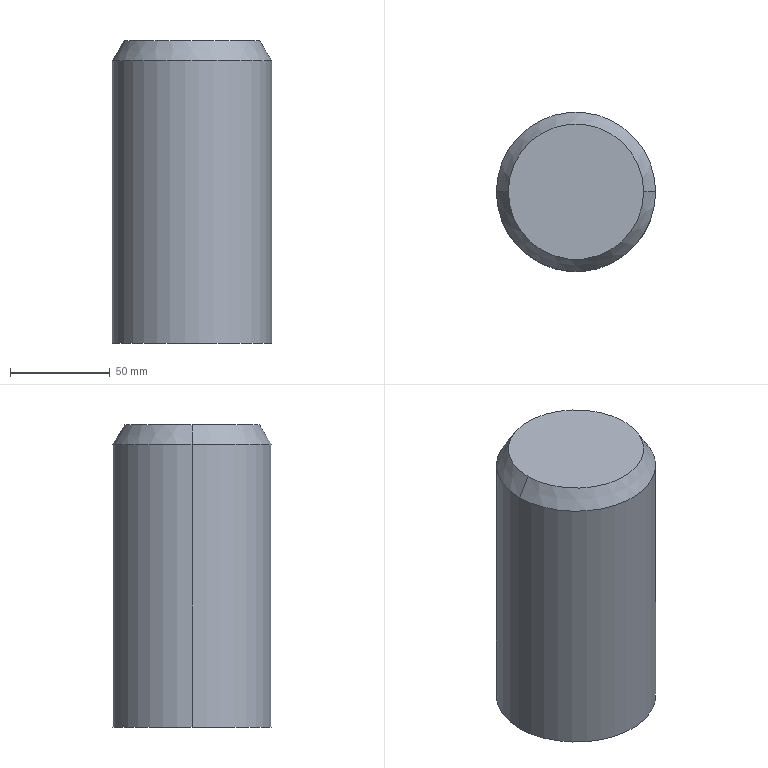Part | SolidWorks | features Chamfer 1, Extrusion 1, HoleWzd 1 | 1 solid | 10 faces | box 80 x 80 x 152 mm | volume 756529 mm3 | cylinder 4 | cone 4 | plane 2 | commonest cylinder face diameters 5 x2 80 x2
STEP:
#1=CARTESIAN_POINT('',(2.5,0.,17.));
#2=VERTEX_POINT('',#1);
#3=CARTESIAN_POINT('',(-2.5,0.,17.));
#4=VERTEX_POINT('',#3);
#5=CARTESIAN_POINT('',(0.,0.,17.));
#6=DIRECTION('',(0.,0.,-1.));
#7=DIRECTION('',(-1.,0.,0.));
#8=AXIS2_PLACEMENT_3D('',#5,#6,#7);
#9=CIRCLE('',#8,2.5);
#10=EDGE_CURVE('',#2,#4,#9,.T.);
#11=ORIENTED_EDGE('',*,*,#10,.F.);
#12=CARTESIAN_POINT('',(2.5,0.,0.));
#13=VERTEX_POINT('',#12);
#14=CARTESIAN_POINT('',(2.5,0.,0.));
#15=DIRECTION('',(0.,0.,-1.));
#16=VECTOR('',#15,1000.);
#17=LINE('',#14,#16);
#18=EDGE_CURVE('',#2,#13,#17,.T.);
#19=ORIENTED_EDGE('',*,*,#18,.T.);
#20=CARTESIAN_POINT('',(-2.5,0.,0.));
#21=VERTEX_POINT('',#20);
#22=CARTESIAN_POINT('',(0.,0.,0.));
#23=DIRECTION('',(0.,0.,-1.));
#24=DIRECTION('',(-1.,0.,0.));
#25=AXIS2_PLACEMENT_3D('',#22,#23,#24);
#26=CIRCLE('',#25,2.5);
#27=EDGE_CURVE('',#13,#21,#26,.T.);
#28=ORIENTED_EDGE('',*,*,#27,.T.);
#29=CARTESIAN_POINT('',(-2.5,0.,0.));
#30=DIRECTION('',(0.,0.,-1.));
#31=VECTOR('',#30,1000.);
#32=LINE('',#29,#31);
#33=EDGE_CURVE('',#4,#21,#32,.T.);
#34=ORIENTED_EDGE('',*,*,#33,.F.);
#35=EDGE_LOOP('',(#11,#19,#28,#34));
#36=FACE_OUTER_BOUND('',#35,.T.);
#37=CARTESIAN_POINT('',(0.,0.,0.));
#38=DIRECTION('',(0.,0.,-1.));
#39=DIRECTION('',(-1.,0.,0.));
#40=AXIS2_PLACEMENT_3D('',#37,#38,#39);
#41=CYLINDRICAL_SURFACE('',#40,2.5);
#42=ADVANCED_FACE('',(#36),#41,.F.);
#43=CARTESIAN_POINT('',(0.,0.,18.502));
#44=VERTEX_POINT('',#43);
#45=CARTESIAN_POINT('',(-2.5,0.,17.));
#46=DIRECTION('',(-0.8572,0.,-0.515));
#47=VECTOR('',#46,1000.);
#48=LINE('',#45,#47);
#49=EDGE_CURVE('',#44,#4,#48,.T.);
#50=ORIENTED_EDGE('',*,*,#49,.F.);
#51=CARTESIAN_POINT('',(2.5,0.,17.));
#52=DIRECTION('',(0.8572,0.,-0.515));
#53=VECTOR('',#52,1000.);
#54=LINE('',#51,#53);
#55=EDGE_CURVE('',#44,#2,#54,.T.);
#56=ORIENTED_EDGE('',*,*,#55,.T.);
#57=ORIENTED_EDGE('',*,*,#10,.T.);
#58=EDGE_LOOP('',(#50,#56,#57));
#59=FACE_OUTER_BOUND('',#58,.T.);
#60=CARTESIAN_POINT('',(0.,0.,17.));
#61=DIRECTION('',(0.,0.,-1.));
#62=DIRECTION('',(-1.,0.,0.));
#63=AXIS2_PLACEMENT_3D('',#60,#61,#62);
#64=CONICAL_SURFACE('',#63,2.5,1.03);
#65=ADVANCED_FACE('',(#59),#64,.F.);
#66=CARTESIAN_POINT('',(34.,0.,152.));
#67=VERTEX_POINT('',#66);
#68=CARTESIAN_POINT('',(-34.,0.,152.));
#69=VERTEX_POINT('',#68);
#70=CARTESIAN_POINT('',(0.,0.,152.));
#71=DIRECTION('',(0.,0.,1.));
#72=DIRECTION('',(1.,0.,0.));
#73=AXIS2_PLACEMENT_3D('',#70,#71,#72);
#74=CIRCLE('',#73,34.);
#75=EDGE_CURVE('',#67,#69,#74,.T.);
#76=ORIENTED_EDGE('',*,*,#75,.F.);
#77=CARTESIAN_POINT('',(40.,0.,142.));
#78=VERTEX_POINT('',#77);
#79=CARTESIAN_POINT('',(34.,0.,152.));
#80=DIRECTION('',(0.5145,0.,-0.8575));
#81=VECTOR('',#80,1000.);
#82=LINE('',#79,#81);
#83=EDGE_CURVE('',#67,#78,#82,.T.);
#84=ORIENTED_EDGE('',*,*,#83,.T.);
#85=CARTESIAN_POINT('',(-40.,0.,142.));
#86=VERTEX_POINT('',#85);
#87=CARTESIAN_POINT('',(0.,0.,142.));
#88=DIRECTION('',(0.,0.,-1.));
#89=DIRECTION('',(1.,0.,0.));
#90=AXIS2_PLACEMENT_3D('',#87,#88,#89);
#91=CIRCLE('',#90,40.);
#92=EDGE_CURVE('',#86,#78,#91,.T.);
#93=ORIENTED_EDGE('',*,*,#92,.F.);
#94=CARTESIAN_POINT('',(-34.,0.,152.));
#95=DIRECTION('',(-0.5145,0.,-0.8575));
#96=VECTOR('',#95,1000.);
#97=LINE('',#94,#96);
#98=EDGE_CURVE('',#69,#86,#97,.T.);
#99=ORIENTED_EDGE('',*,*,#98,.F.);
#100=EDGE_LOOP('',(#76,#84,#93,#99));
#101=FACE_OUTER_BOUND('',#100,.T.);
#102=CARTESIAN_POINT('',(0.,0.,152.));
#103=DIRECTION('',(0.,0.,-1.));
#104=DIRECTION('',(-1.,0.,0.));
#105=AXIS2_PLACEMENT_3D('',#102,#103,#104);
#106=CONICAL_SURFACE('',#105,34.,0.5404);
#107=ADVANCED_FACE('',(#101),#106,.T.);
#108=ORIENTED_EDGE('',*,*,#92,.T.);
#109=CARTESIAN_POINT('',(40.,0.,0.));
#110=VERTEX_POINT('',#109);
#111=CARTESIAN_POINT('',(40.,0.,152.));
#112=DIRECTION('',(0.,0.,-1.));
#113=VECTOR('',#112,1000.);
#114=LINE('',#111,#113);
#115=EDGE_CURVE('',#78,#110,#114,.T.);
#116=ORIENTED_EDGE('',*,*,#115,.T.);
#117=CARTESIAN_POINT('',(-40.,0.,0.));
#118=VERTEX_POINT('',#117);
#119=CARTESIAN_POINT('',(0.,0.,0.));
#120=DIRECTION('',(0.,0.,1.));
#121=DIRECTION('',(1.,0.,0.));
#122=AXIS2_PLACEMENT_3D('',#119,#120,#121);
#123=CIRCLE('',#122,40.);
#124=EDGE_CURVE('',#110,#118,#123,.T.);
#125=ORIENTED_EDGE('',*,*,#124,.T.);
#126=CARTESIAN_POINT('',(-40.,0.,152.));
#127=DIRECTION('',(0.,0.,-1.));
#128=VECTOR('',#127,1000.);
#129=LINE('',#126,#128);
#130=EDGE_CURVE('',#86,#118,#129,.T.);
#131=ORIENTED_EDGE('',*,*,#130,.F.);
#132=EDGE_LOOP('',(#108,#116,#125,#131));
#133=FACE_OUTER_BOUND('',#132,.T.);
#134=CARTESIAN_POINT('',(0.,0.,152.));
#135=DIRECTION('',(0.,0.,-1.));
#136=DIRECTION('',(-1.,0.,0.));
#137=AXIS2_PLACEMENT_3D('',#134,#135,#136);
#138=CYLINDRICAL_SURFACE('',#137,40.);
#139=ADVANCED_FACE('',(#133),#138,.T.);
#140=CARTESIAN_POINT('',(0.,0.,0.));
#141=DIRECTION('',(0.,0.,1.));
#142=DIRECTION('',(1.,0.,0.));
#143=AXIS2_PLACEMENT_3D('',#140,#141,#142);
#144=CIRCLE('',#143,40.);
#145=EDGE_CURVE('',#118,#110,#144,.T.);
#146=ORIENTED_EDGE('',*,*,#145,.F.);
#147=ORIENTED_EDGE('',*,*,#124,.F.);
#148=EDGE_LOOP('',(#146,#147));
#149=FACE_OUTER_BOUND('',#148,.T.);
#150=CARTESIAN_POINT('',(0.,0.,0.));
#151=DIRECTION('',(0.,0.,-1.));
#152=DIRECTION('',(-1.,0.,0.));
#153=AXIS2_PLACEMENT_3D('',#150,#151,#152);
#154=CIRCLE('',#153,2.5);
#155=EDGE_CURVE('',#21,#13,#154,.T.);
#156=ORIENTED_EDGE('',*,*,#155,.F.);
#157=ORIENTED_EDGE('',*,*,#27,.F.);
#158=EDGE_LOOP('',(#156,#157));
#159=FACE_BOUND('',#158,.T.);
#160=CARTESIAN_POINT('',(0.,0.,0.));
#161=DIRECTION('',(0.,0.,1.));
#162=DIRECTION('',(1.,0.,0.));
#163=AXIS2_PLACEMENT_3D('',#160,#161,#162);
#164=PLANE('',#163);
#165=ADVANCED_FACE('',(#149,#159),#164,.F.);
#166=ORIENTED_EDGE('',*,*,#115,.F.);
#167=CARTESIAN_POINT('',(0.,0.,142.));
#168=DIRECTION('',(0.,0.,-1.));
#169=DIRECTION('',(1.,0.,0.));
#170=AXIS2_PLACEMENT_3D('',#167,#168,#169);
#171=CIRCLE('',#170,40.);
#172=EDGE_CURVE('',#78,#86,#171,.T.);
#173=ORIENTED_EDGE('',*,*,#172,.T.);
#174=ORIENTED_EDGE('',*,*,#130,.T.);
#175=ORIENTED_EDGE('',*,*,#145,.T.);
#176=EDGE_LOOP('',(#166,#173,#174,#175));
#177=FACE_OUTER_BOUND('',#176,.T.);
#178=CARTESIAN_POINT('',(0.,0.,152.));
#179=DIRECTION('',(0.,0.,-1.));
#180=DIRECTION('',(-1.,0.,0.));
#181=AXIS2_PLACEMENT_3D('',#178,#179,#180);
#182=CYLINDRICAL_SURFACE('',#181,40.);
#183=ADVANCED_FACE('',(#177),#182,.T.);
#184=CARTESIAN_POINT('',(0.,0.,152.));
#185=DIRECTION('',(0.,0.,1.));
#186=DIRECTION('',(1.,0.,0.));
#187=AXIS2_PLACEMENT_3D('',#184,#185,#186);
#188=CIRCLE('',#187,34.);
#189=EDGE_CURVE('',#69,#67,#188,.T.);
#190=ORIENTED_EDGE('',*,*,#189,.T.);
#191=ORIENTED_EDGE('',*,*,#75,.T.);
#192=EDGE_LOOP('',(#190,#191));
#193=FACE_OUTER_BOUND('',#192,.T.);
#194=CARTESIAN_POINT('',(0.,0.,152.));
#195=DIRECTION('',(0.,0.,1.));
#196=DIRECTION('',(1.,0.,0.));
#197=AXIS2_PLACEMENT_3D('',#194,#195,#196);
#198=PLANE('',#197);
#199=ADVANCED_FACE('',(#193),#198,.T.);
#200=ORIENTED_EDGE('',*,*,#83,.F.);
#201=ORIENTED_EDGE('',*,*,#189,.F.);
#202=ORIENTED_EDGE('',*,*,#98,.T.);
#203=ORIENTED_EDGE('',*,*,#172,.F.);
#204=EDGE_LOOP('',(#200,#201,#202,#203));
#205=FACE_OUTER_BOUND('',#204,.T.);
#206=CARTESIAN_POINT('',(0.,0.,152.));
#207=DIRECTION('',(0.,0.,-1.));
#208=DIRECTION('',(-1.,0.,0.));
#209=AXIS2_PLACEMENT_3D('',#206,#207,#208);
#210=CONICAL_SURFACE('',#209,34.,0.5404);
#211=ADVANCED_FACE('',(#205),#210,.T.);
#212=ORIENTED_EDGE('',*,*,#55,.F.);
#213=ORIENTED_EDGE('',*,*,#49,.T.);
#214=CARTESIAN_POINT('',(0.,0.,17.));
#215=DIRECTION('',(0.,0.,-1.));
#216=DIRECTION('',(-1.,0.,0.));
#217=AXIS2_PLACEMENT_3D('',#214,#215,#216);
#218=CIRCLE('',#217,2.5);
#219=EDGE_CURVE('',#4,#2,#218,.T.);
#220=ORIENTED_EDGE('',*,*,#219,.T.);
#221=EDGE_LOOP('',(#212,#213,#220));
#222=FACE_OUTER_BOUND('',#221,.T.);
#223=CARTESIAN_POINT('',(0.,0.,17.));
#224=DIRECTION('',(0.,0.,-1.));
#225=DIRECTION('',(-1.,0.,0.));
#226=AXIS2_PLACEMENT_3D('',#223,#224,#225);
#227=CONICAL_SURFACE('',#226,2.5,1.03);
#228=ADVANCED_FACE('',(#222),#227,.F.);
#229=ORIENTED_EDGE('',*,*,#18,.F.);
#230=ORIENTED_EDGE('',*,*,#219,.F.);
#231=ORIENTED_EDGE('',*,*,#33,.T.);
#232=ORIENTED_EDGE('',*,*,#155,.T.);
#233=EDGE_LOOP('',(#229,#230,#231,#232));
#234=FACE_OUTER_BOUND('',#233,.T.);
#235=CARTESIAN_POINT('',(0.,0.,0.));
#236=DIRECTION('',(0.,0.,-1.));
#237=DIRECTION('',(-1.,0.,0.));
#238=AXIS2_PLACEMENT_3D('',#235,#236,#237);
#239=CYLINDRICAL_SURFACE('',#238,2.5);
#240=ADVANCED_FACE('',(#234),#239,.F.);
#241=CLOSED_SHELL('',(#42,#65,#107,#139,#165,#183,#199,#211,#228,#240));
#242=MANIFOLD_SOLID_BREP('',#241);
#243=CARTESIAN_POINT('',(0.,0.,0.));
#244=DIRECTION('',(0.,0.,1.));
#245=DIRECTION('',(1.,0.,0.));
#246=AXIS2_PLACEMENT_3D('',#243,#244,#245);
#247=(LENGTH_UNIT()NAMED_UNIT(*)SI_UNIT(.MILLI.,.METRE.));
#248=UNCERTAINTY_MEASURE_WITH_UNIT(LENGTH_MEASURE(0.00001),#247,'','');
#249=(NAMED_UNIT(*)PLANE_ANGLE_UNIT()SI_UNIT($,.RADIAN.));
#250=(NAMED_UNIT(*)SI_UNIT($,.STERADIAN.)SOLID_ANGLE_UNIT());
#251=(GEOMETRIC_REPRESENTATION_CONTEXT(3)GLOBAL_UNCERTAINTY_ASSIGNED_CONTEXT((#248))GLOBAL_UNIT_ASSIGNED_CONTEXT((#247,#249,#250))REPRESENTATION_CONTEXT('',''));
#252=ADVANCED_BREP_SHAPE_REPRESENTATION('',(#242,#246),#251);